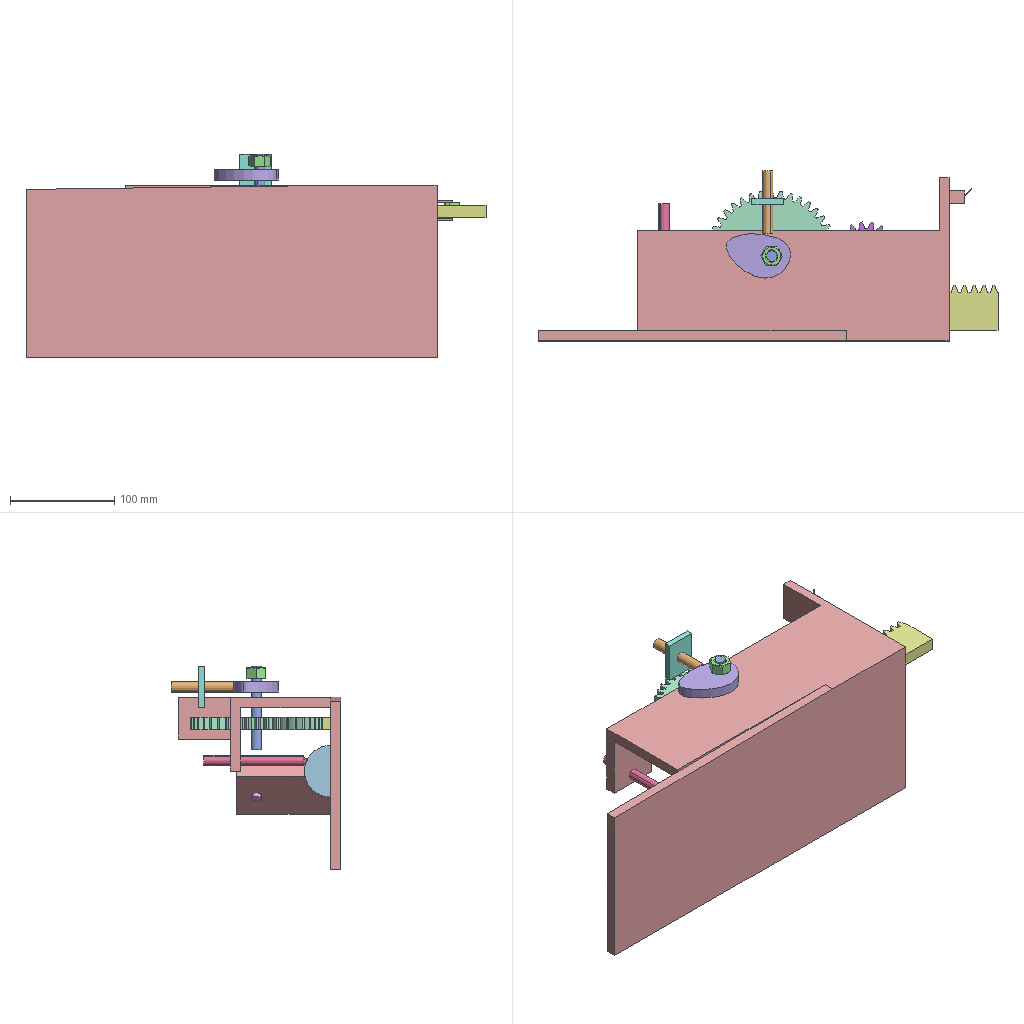Assembly | SolidWorks | 15 different items | 15 placed | box 441 x 163 x 195 mm
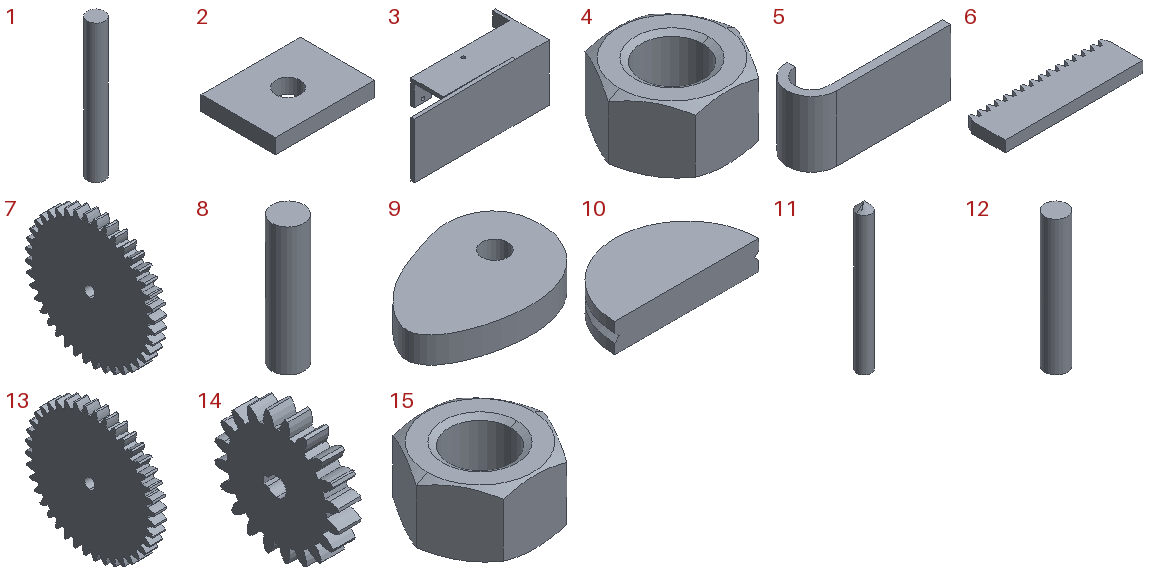Parts list (item | quantity | size | volume | features):
1 | x1 | 10 x 10 x 80 mm | 6158 mm3 | features Extrusion 1, ICE 1
2 | x1 | 40 x 30 x 6 mm | 6729 mm3 | features Extrusion 1, ICE 1
3 | x1 | 408.883 x 156 x 165.33 mm | 1077828 mm3 | features ICE 36, Extrusion 1, Sweep 1
4 | x1 | 20.785 x 18 x 10.8 mm | 2118 mm3 | features BaseBody 1
5 | x1 | 17 x 6 x 8 mm | 174.832 mm3 | features Extrusion 1
6 | x1 | 150 x 43 x 12 mm | 70879 mm3 | features BaseBody 1
7 | x1 | 12 x 125.745 x 125.745 mm | 132575 mm3 | features Boss 3, Cut 3, CirPattern 2, Fillet 2, Revolution 1
8 | x1 | 10 x 10 x 40 mm | 3009 mm3 | features Extrusion 1, ICE 1
9 | x1 | 60.725 x 43.378 x 10 mm | 18972 mm3 | features Extrusion 1
10 | x1 | 50 x 25 x 10 mm | 9644 mm3 | features Extrusion 1, SweepCut 1
11 | x1 | 10 x 10 x 100 mm | 7592 mm3 | features Chamfer 1, Extrusion 1
12 | x1 | 10 x 10 x 60 mm | 4712 mm3 | features Extrusion 1
13 | x1 | 12 x 125.745 x 125.745 mm | 132575 mm3 | features BaseBody 1
14 | x1 | 12 x 65.416 x 65.416 mm | 31703 mm3 | features BaseBody 1
15 | x1 | 20.785 x 18 x 10.8 mm | 2118 mm3 | features RevCut 2, Chamfer 1, Extrusion 1, LPattern 1
Mates (type | each side: item.copy, entity, surface, feature):
Concentric | 3.1 face cylinder Cut-Extrude24 | 1.1 face cylinder Boss-Extrude1
Symmetric | 3.1 face plane Boss-Extrude4 | 1.1 face plane Boss-Extrude1 | 1.1 face plane Boss-Extrude1
Hinge | 3.1 face cylinder Boss-Extrude11 | 5.1 face cylinder Boss-Extrude1 | 3.1 face plane Boss-Extrude10 | 5.1 face plane Boss-Extrude1
LimitPlanarAngleDim | 5.1 face plane Boss-Extrude1 | 3.1 face plane Cut-Extrude4
Concentric | 3.1 face cylinder Cut-Extrude29 | 8.1 face cylinder Boss-Extrude1
DistanceDim | 8.1 face plane Boss-Extrude1 | 3.1 face plane Boss-Extrude22
UniversalJoint | 1.1 face cylinder Boss-Extrude1 | 8.1 face cylinder Boss-Extrude1
Parallel | 3.1 face plane Boss-Extrude1 | 2.1 face plane Boss-Extrude1
Coincident | 3.1 face plane Boss-Extrude4 | 2.1 face plane Boss-Extrude1
Concentric | 2.1 face cylinder Cut-Extrude1 | 12.1 face cylinder Boss-Extrude1
Concentric | 1.1 face cylinder Boss-Extrude1 | 9.1 face cylinder Boss-Extrude1
Lock | 1.1 select_type:0 | 9.1 select_type:0
CamTangent | 9.1 face surface:4009 Boss-Extrude1 | 12.1 face plane Boss-Extrude1
Concentric | 4.1 face cylinder Input1 | 1.1 face cylinder Boss-Extrude1
Screw | 1.1 face cylinder Boss-Extrude1 | 4.1 edge
Concentric | 3.1 face cylinder Cut-Extrude26 | 11.1 face cylinder Boss-Extrude1
Coincident | 3.1 face plane Boss-Extrude13 | 10.1 face plane Boss-Extrude1
Perpendicular | 3.1 face plane Boss-Extrude4 | 10.1 edge
Path | 11.1 vertex | 10.1 edge
Coincident | 3.1 face plane Boss-Extrude13 | 6.1 face plane Input1
Concentric | 3.1 face cylinder Boss-Extrude2 | 14.1 face cylinder Input1
DistanceDim | 3.1 face plane Cut-Extrude7 | 14.1 face plane Input1
RackPinionDim | 6.1 edge | 14.1 edge
Coincident | 6.1 face plane Input1 | 14.1 face plane Input1
Concentric | 1.1 face cylinder Boss-Extrude1 | 13.1 face cylinder Input1
GearDim | 14.1 edge | 13.1 edge
Lock | 1.1 select_type:0 | 13.1 select_type:0
LimitDistanceDim | 6.1 face plane Input1 | 3.1 face plane Cut-Extrude4